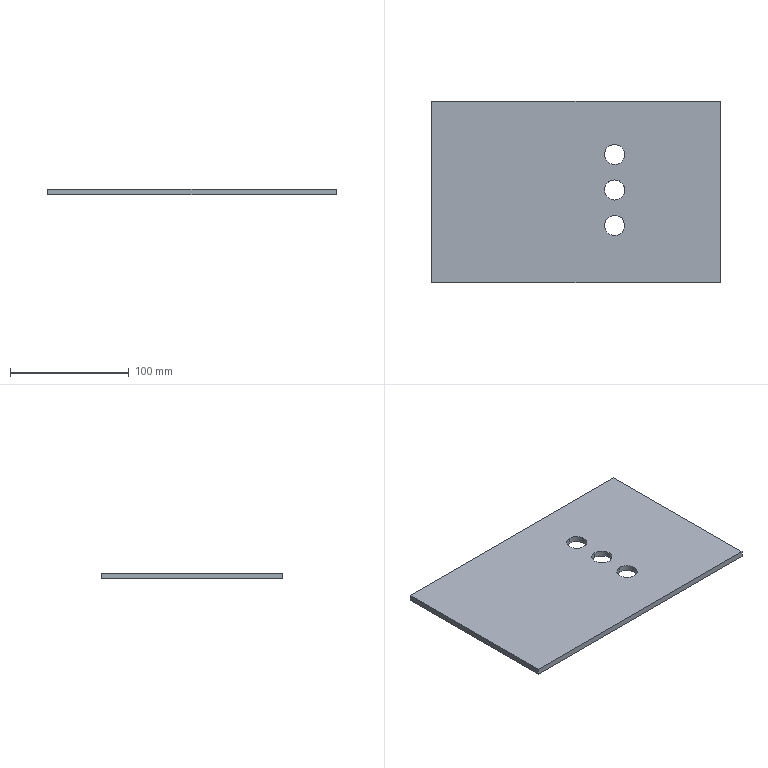Part | NX | features BREP 1 | 1 solid | 12 faces | box 243.374 x 152.848 x 5 mm | volume 182593 mm3 | cylinder 6 | plane 6 | commonest cylinder face diameters 17 x6
STEP:
#1=CARTESIAN_POINT('',(1894.999,-438.5,55.));
#2=VERTEX_POINT('',#1);
#3=CARTESIAN_POINT('',(1895.001,-421.5,55.));
#4=VERTEX_POINT('',#3);
#5=CARTESIAN_POINT('',(1895.,-438.5,55.));
#6=CARTESIAN_POINT('',(1895.974,-438.5,55.));
#7=CARTESIAN_POINT('',(1897.93,-438.172,55.));
#8=CARTESIAN_POINT('',(1901.646,-436.045,55.));
#9=CARTESIAN_POINT('',(1904.44,-430.737,55.));
#10=CARTESIAN_POINT('',(1902.023,-423.576,55.));
#11=CARTESIAN_POINT('',(1897.362,-421.5,55.));
#12=CARTESIAN_POINT('',(1895.001,-421.5,55.));
#13=B_SPLINE_CURVE_WITH_KNOTS('',3,(#5,#6,#7,#8,#9,#10,#11,#12),.UNSPECIFIED.,.F.,.F.,(4,1,1,1,1,4),(0.,0.125,0.25,0.5,0.75,1.),.UNSPECIFIED.);
#14=EDGE_CURVE('',#2,#4,#13,.T.);
#15=ORIENTED_EDGE('',*,*,#14,.F.);
#16=CARTESIAN_POINT('',(1895.001,-438.5,60.));
#17=VERTEX_POINT('',#16);
#18=CARTESIAN_POINT('',(1895.,-438.5,55.));
#19=CARTESIAN_POINT('',(1895.,-438.5,56.));
#20=CARTESIAN_POINT('',(1895.,-438.5,57.));
#21=CARTESIAN_POINT('',(1895.,-438.5,58.));
#22=CARTESIAN_POINT('',(1895.,-438.5,59.));
#23=CARTESIAN_POINT('',(1895.,-438.5,60.));
#24=(BOUNDED_CURVE()B_SPLINE_CURVE(5,(#18,#19,#20,#21,#22,#23),.UNSPECIFIED.,.F.,.F.)B_SPLINE_CURVE_WITH_KNOTS((6,6),(106.,111.),.UNSPECIFIED.)CURVE()GEOMETRIC_REPRESENTATION_ITEM()RATIONAL_B_SPLINE_CURVE((1.,1.,1.,1.,1.,1.))REPRESENTATION_ITEM(''));
#25=EDGE_CURVE('',#2,#17,#24,.T.);
#26=ORIENTED_EDGE('',*,*,#25,.T.);
#27=CARTESIAN_POINT('',(1894.999,-421.5,60.));
#28=VERTEX_POINT('',#27);
#29=CARTESIAN_POINT('',(1895.,-421.5,60.));
#30=CARTESIAN_POINT('',(1897.359,-421.5,60.));
#31=CARTESIAN_POINT('',(1902.023,-423.576,60.));
#32=CARTESIAN_POINT('',(1904.44,-430.736,60.));
#33=CARTESIAN_POINT('',(1901.647,-436.044,60.));
#34=CARTESIAN_POINT('',(1897.931,-438.171,60.));
#35=CARTESIAN_POINT('',(1895.976,-438.5,60.));
#36=CARTESIAN_POINT('',(1895.001,-438.5,60.));
#37=B_SPLINE_CURVE_WITH_KNOTS('',3,(#29,#30,#31,#32,#33,#34,#35,#36),.UNSPECIFIED.,.F.,.F.,(4,1,1,1,1,4),(0.,0.25,0.5,0.75,0.875,1.),.UNSPECIFIED.);
#38=EDGE_CURVE('',#17,#28,#37,.F.);
#39=ORIENTED_EDGE('',*,*,#38,.T.);
#40=CARTESIAN_POINT('',(1895.,-421.5,55.));
#41=CARTESIAN_POINT('',(1895.,-421.5,56.));
#42=CARTESIAN_POINT('',(1895.,-421.5,57.));
#43=CARTESIAN_POINT('',(1895.,-421.5,58.));
#44=CARTESIAN_POINT('',(1895.,-421.5,59.));
#45=CARTESIAN_POINT('',(1895.,-421.5,60.));
#46=(BOUNDED_CURVE()B_SPLINE_CURVE(5,(#40,#41,#42,#43,#44,#45),.UNSPECIFIED.,.F.,.F.)B_SPLINE_CURVE_WITH_KNOTS((6,6),(106.,111.),.UNSPECIFIED.)CURVE()GEOMETRIC_REPRESENTATION_ITEM()RATIONAL_B_SPLINE_CURVE((0.25,0.25,0.25,0.25,0.25,0.25))REPRESENTATION_ITEM(''));
#47=EDGE_CURVE('',#4,#28,#46,.T.);
#48=ORIENTED_EDGE('',*,*,#47,.F.);
#49=EDGE_LOOP('',(#15,#26,#39,#48));
#50=FACE_BOUND('',#49,.T.);
#51=CARTESIAN_POINT('',(1895.,-430.,49.));
#52=DIRECTION('',(0.,0.,1.));
#53=DIRECTION('',(1.,0.,0.));
#54=AXIS2_PLACEMENT_3D('',#51,#52,#53);
#55=CYLINDRICAL_SURFACE('',#54,8.5);
#56=ADVANCED_FACE('',(#50),#55,.F.);
#57=CARTESIAN_POINT('',(1895.,-421.5,55.));
#58=CARTESIAN_POINT('',(1892.641,-421.5,55.));
#59=CARTESIAN_POINT('',(1887.977,-423.575,55.));
#60=CARTESIAN_POINT('',(1885.56,-430.735,55.));
#61=CARTESIAN_POINT('',(1888.352,-436.043,55.));
#62=CARTESIAN_POINT('',(1892.069,-438.171,55.));
#63=CARTESIAN_POINT('',(1894.024,-438.5,55.));
#64=CARTESIAN_POINT('',(1894.999,-438.5,55.));
#65=B_SPLINE_CURVE_WITH_KNOTS('',3,(#57,#58,#59,#60,#61,#62,#63,#64),.UNSPECIFIED.,.F.,.F.,(4,1,1,1,1,4),(0.,0.25,0.5,0.75,0.875,1.),.UNSPECIFIED.);
#66=EDGE_CURVE('',#4,#2,#65,.T.);
#67=ORIENTED_EDGE('',*,*,#66,.F.);
#68=ORIENTED_EDGE('',*,*,#47,.T.);
#69=CARTESIAN_POINT('',(1895.,-438.5,60.));
#70=CARTESIAN_POINT('',(1894.026,-438.5,60.));
#71=CARTESIAN_POINT('',(1892.069,-438.172,60.));
#72=CARTESIAN_POINT('',(1888.353,-436.044,60.));
#73=CARTESIAN_POINT('',(1885.56,-430.737,60.));
#74=CARTESIAN_POINT('',(1887.977,-423.576,60.));
#75=CARTESIAN_POINT('',(1892.639,-421.5,60.));
#76=CARTESIAN_POINT('',(1894.999,-421.5,60.));
#77=B_SPLINE_CURVE_WITH_KNOTS('',3,(#69,#70,#71,#72,#73,#74,#75,#76),.UNSPECIFIED.,.F.,.F.,(4,1,1,1,1,4),(0.,0.125,0.25,0.5,0.75,1.),.UNSPECIFIED.);
#78=EDGE_CURVE('',#28,#17,#77,.F.);
#79=ORIENTED_EDGE('',*,*,#78,.T.);
#80=ORIENTED_EDGE('',*,*,#25,.F.);
#81=EDGE_LOOP('',(#67,#68,#79,#80));
#82=FACE_BOUND('',#81,.T.);
#83=CARTESIAN_POINT('',(1895.,-430.,49.));
#84=DIRECTION('',(0.,0.,1.));
#85=DIRECTION('',(0.,-1.,0.));
#86=AXIS2_PLACEMENT_3D('',#83,#84,#85);
#87=CYLINDRICAL_SURFACE('',#86,8.5);
#88=ADVANCED_FACE('',(#82),#87,.F.);
#89=CARTESIAN_POINT('',(1894.999,-468.5,55.));
#90=VERTEX_POINT('',#89);
#91=CARTESIAN_POINT('',(1895.001,-451.5,55.));
#92=VERTEX_POINT('',#91);
#93=CARTESIAN_POINT('',(1895.,-468.5,55.));
#94=CARTESIAN_POINT('',(1895.974,-468.5,55.));
#95=CARTESIAN_POINT('',(1897.93,-468.172,55.));
#96=CARTESIAN_POINT('',(1901.646,-466.045,55.));
#97=CARTESIAN_POINT('',(1904.44,-460.737,55.));
#98=CARTESIAN_POINT('',(1902.023,-453.576,55.));
#99=CARTESIAN_POINT('',(1897.362,-451.5,55.));
#100=CARTESIAN_POINT('',(1895.001,-451.5,55.));
#101=B_SPLINE_CURVE_WITH_KNOTS('',3,(#93,#94,#95,#96,#97,#98,#99,#100),.UNSPECIFIED.,.F.,.F.,(4,1,1,1,1,4),(0.,0.125,0.25,0.5,0.75,1.),.UNSPECIFIED.);
#102=EDGE_CURVE('',#90,#92,#101,.T.);
#103=ORIENTED_EDGE('',*,*,#102,.F.);
#104=CARTESIAN_POINT('',(1895.001,-468.5,60.));
#105=VERTEX_POINT('',#104);
#106=CARTESIAN_POINT('',(1895.,-468.5,55.));
#107=CARTESIAN_POINT('',(1895.,-468.5,56.));
#108=CARTESIAN_POINT('',(1895.,-468.5,57.));
#109=CARTESIAN_POINT('',(1895.,-468.5,58.));
#110=CARTESIAN_POINT('',(1895.,-468.5,59.));
#111=CARTESIAN_POINT('',(1895.,-468.5,60.));
#112=(BOUNDED_CURVE()B_SPLINE_CURVE(5,(#106,#107,#108,#109,#110,#111),.UNSPECIFIED.,.F.,.F.)B_SPLINE_CURVE_WITH_KNOTS((6,6),(106.,111.),.UNSPECIFIED.)CURVE()GEOMETRIC_REPRESENTATION_ITEM()RATIONAL_B_SPLINE_CURVE((1.,1.,1.,1.,1.,1.))REPRESENTATION_ITEM(''));
#113=EDGE_CURVE('',#90,#105,#112,.T.);
#114=ORIENTED_EDGE('',*,*,#113,.T.);
#115=CARTESIAN_POINT('',(1894.999,-451.5,60.));
#116=VERTEX_POINT('',#115);
#117=CARTESIAN_POINT('',(1895.,-451.5,60.));
#118=CARTESIAN_POINT('',(1897.359,-451.5,60.));
#119=CARTESIAN_POINT('',(1902.023,-453.576,60.));
#120=CARTESIAN_POINT('',(1904.44,-460.736,60.));
#121=CARTESIAN_POINT('',(1901.647,-466.044,60.));
#122=CARTESIAN_POINT('',(1897.931,-468.171,60.));
#123=CARTESIAN_POINT('',(1895.976,-468.5,60.));
#124=CARTESIAN_POINT('',(1895.001,-468.5,60.));
#125=B_SPLINE_CURVE_WITH_KNOTS('',3,(#117,#118,#119,#120,#121,#122,#123,#124),.UNSPECIFIED.,.F.,.F.,(4,1,1,1,1,4),(0.,0.25,0.5,0.75,0.875,1.),.UNSPECIFIED.);
#126=EDGE_CURVE('',#105,#116,#125,.F.);
#127=ORIENTED_EDGE('',*,*,#126,.T.);
#128=CARTESIAN_POINT('',(1895.,-451.5,55.));
#129=CARTESIAN_POINT('',(1895.,-451.5,56.));
#130=CARTESIAN_POINT('',(1895.,-451.5,57.));
#131=CARTESIAN_POINT('',(1895.,-451.5,58.));
#132=CARTESIAN_POINT('',(1895.,-451.5,59.));
#133=CARTESIAN_POINT('',(1895.,-451.5,60.));
#134=(BOUNDED_CURVE()B_SPLINE_CURVE(5,(#128,#129,#130,#131,#132,#133),.UNSPECIFIED.,.F.,.F.)B_SPLINE_CURVE_WITH_KNOTS((6,6),(106.,111.),.UNSPECIFIED.)CURVE()GEOMETRIC_REPRESENTATION_ITEM()RATIONAL_B_SPLINE_CURVE((0.25,0.25,0.25,0.25,0.25,0.25))REPRESENTATION_ITEM(''));
#135=EDGE_CURVE('',#92,#116,#134,.T.);
#136=ORIENTED_EDGE('',*,*,#135,.F.);
#137=EDGE_LOOP('',(#103,#114,#127,#136));
#138=FACE_BOUND('',#137,.T.);
#139=CARTESIAN_POINT('',(1895.,-460.,49.));
#140=DIRECTION('',(0.,0.,1.));
#141=DIRECTION('',(1.,0.,0.));
#142=AXIS2_PLACEMENT_3D('',#139,#140,#141);
#143=CYLINDRICAL_SURFACE('',#142,8.5);
#144=ADVANCED_FACE('',(#138),#143,.F.);
#145=CARTESIAN_POINT('',(1895.,-451.5,55.));
#146=CARTESIAN_POINT('',(1892.641,-451.5,55.));
#147=CARTESIAN_POINT('',(1887.977,-453.575,55.));
#148=CARTESIAN_POINT('',(1885.56,-460.735,55.));
#149=CARTESIAN_POINT('',(1888.352,-466.043,55.));
#150=CARTESIAN_POINT('',(1892.069,-468.171,55.));
#151=CARTESIAN_POINT('',(1894.024,-468.5,55.));
#152=CARTESIAN_POINT('',(1894.999,-468.5,55.));
#153=B_SPLINE_CURVE_WITH_KNOTS('',3,(#145,#146,#147,#148,#149,#150,#151,#152),.UNSPECIFIED.,.F.,.F.,(4,1,1,1,1,4),(0.,0.25,0.5,0.75,0.875,1.),.UNSPECIFIED.);
#154=EDGE_CURVE('',#92,#90,#153,.T.);
#155=ORIENTED_EDGE('',*,*,#154,.F.);
#156=ORIENTED_EDGE('',*,*,#135,.T.);
#157=CARTESIAN_POINT('',(1895.,-468.5,60.));
#158=CARTESIAN_POINT('',(1894.026,-468.5,60.));
#159=CARTESIAN_POINT('',(1892.069,-468.172,60.));
#160=CARTESIAN_POINT('',(1888.353,-466.044,60.));
#161=CARTESIAN_POINT('',(1885.56,-460.737,60.));
#162=CARTESIAN_POINT('',(1887.977,-453.576,60.));
#163=CARTESIAN_POINT('',(1892.639,-451.5,60.));
#164=CARTESIAN_POINT('',(1894.999,-451.5,60.));
#165=B_SPLINE_CURVE_WITH_KNOTS('',3,(#157,#158,#159,#160,#161,#162,#163,#164),.UNSPECIFIED.,.F.,.F.,(4,1,1,1,1,4),(0.,0.125,0.25,0.5,0.75,1.),.UNSPECIFIED.);
#166=EDGE_CURVE('',#116,#105,#165,.F.);
#167=ORIENTED_EDGE('',*,*,#166,.T.);
#168=ORIENTED_EDGE('',*,*,#113,.F.);
#169=EDGE_LOOP('',(#155,#156,#167,#168));
#170=FACE_BOUND('',#169,.T.);
#171=CARTESIAN_POINT('',(1895.,-460.,49.));
#172=DIRECTION('',(0.,0.,1.));
#173=DIRECTION('',(0.,-1.,0.));
#174=AXIS2_PLACEMENT_3D('',#171,#172,#173);
#175=CYLINDRICAL_SURFACE('',#174,8.5);
#176=ADVANCED_FACE('',(#170),#175,.F.);
#177=CARTESIAN_POINT('',(1894.999,-498.5,55.));
#178=VERTEX_POINT('',#177);
#179=CARTESIAN_POINT('',(1895.001,-481.5,55.));
#180=VERTEX_POINT('',#179);
#181=CARTESIAN_POINT('',(1895.,-498.5,55.));
#182=CARTESIAN_POINT('',(1895.974,-498.5,55.));
#183=CARTESIAN_POINT('',(1897.93,-498.172,55.));
#184=CARTESIAN_POINT('',(1901.646,-496.045,55.));
#185=CARTESIAN_POINT('',(1904.44,-490.737,55.));
#186=CARTESIAN_POINT('',(1902.023,-483.576,55.));
#187=CARTESIAN_POINT('',(1897.362,-481.5,55.));
#188=CARTESIAN_POINT('',(1895.001,-481.5,55.));
#189=B_SPLINE_CURVE_WITH_KNOTS('',3,(#181,#182,#183,#184,#185,#186,#187,#188),.UNSPECIFIED.,.F.,.F.,(4,1,1,1,1,4),(0.,0.125,0.25,0.5,0.75,1.),.UNSPECIFIED.);
#190=EDGE_CURVE('',#178,#180,#189,.T.);
#191=ORIENTED_EDGE('',*,*,#190,.F.);
#192=CARTESIAN_POINT('',(1895.,-498.5,60.));
#193=VERTEX_POINT('',#192);
#194=CARTESIAN_POINT('',(1895.,-498.5,55.));
#195=CARTESIAN_POINT('',(1895.,-498.5,56.));
#196=CARTESIAN_POINT('',(1895.,-498.5,57.));
#197=CARTESIAN_POINT('',(1895.,-498.5,58.));
#198=CARTESIAN_POINT('',(1895.,-498.5,59.));
#199=CARTESIAN_POINT('',(1895.,-498.5,60.));
#200=(BOUNDED_CURVE()B_SPLINE_CURVE(5,(#194,#195,#196,#197,#198,#199),.UNSPECIFIED.,.F.,.F.)B_SPLINE_CURVE_WITH_KNOTS((6,6),(106.,111.),.UNSPECIFIED.)CURVE()GEOMETRIC_REPRESENTATION_ITEM()RATIONAL_B_SPLINE_CURVE((1.,1.,1.,1.,1.,1.))REPRESENTATION_ITEM(''));
#201=EDGE_CURVE('',#178,#193,#200,.T.);
#202=ORIENTED_EDGE('',*,*,#201,.T.);
#203=CARTESIAN_POINT('',(1895.,-481.5,60.));
#204=VERTEX_POINT('',#203);
#205=CARTESIAN_POINT('',(1895.,-498.5,60.));
#206=CARTESIAN_POINT('',(1895.807,-498.5,60.));
#207=CARTESIAN_POINT('',(1896.636,-498.404,60.));
#208=CARTESIAN_POINT('',(1897.469,-498.202,60.));
#209=CARTESIAN_POINT('',(1899.048,-497.596,60.));
#210=CARTESIAN_POINT('',(1900.474,-496.585,60.));
#211=CARTESIAN_POINT('',(1901.109,-496.004,60.));
#212=CARTESIAN_POINT('',(1902.209,-494.702,60.));
#213=CARTESIAN_POINT('',(1902.968,-493.138,60.));
#214=CARTESIAN_POINT('',(1903.245,-492.321,60.));
#215=CARTESIAN_POINT('',(1903.584,-490.642,60.));
#216=CARTESIAN_POINT('',(1903.495,-488.91,60.));
#217=CARTESIAN_POINT('',(1903.343,-488.06,60.));
#218=CARTESIAN_POINT('',(1902.828,-486.42,60.));
#219=CARTESIAN_POINT('',(1901.916,-484.948,60.));
#220=CARTESIAN_POINT('',(1901.371,-484.276,60.));
#221=CARTESIAN_POINT('',(1900.125,-483.084,60.));
#222=CARTESIAN_POINT('',(1898.617,-482.236,60.));
#223=CARTESIAN_POINT('',(1897.815,-481.911,60.));
#224=CARTESIAN_POINT('',(1896.759,-481.631,60.));
#225=CARTESIAN_POINT('',(1895.679,-481.523,60.));
#226=CARTESIAN_POINT('',(1895.453,-481.508,60.));
#227=CARTESIAN_POINT('',(1895.227,-481.5,60.));
#228=CARTESIAN_POINT('',(1895.,-481.5,60.));
#229=B_SPLINE_CURVE_WITH_KNOTS('',5,(#205,#206,#207,#208,#209,#210,#211,#212,#213,#214,#215,#216,#217,#218,#219,#220,#221,#222,#223,#224,#225,#226,#227,#228),.UNSPECIFIED.,.F.,.F.,(6,3,3,3,3,3,3,6),(0.,6.667,12.918,18.932,24.809,30.609,36.373,37.896),.UNSPECIFIED.);
#230=EDGE_CURVE('',#193,#204,#229,.T.);
#231=ORIENTED_EDGE('',*,*,#230,.T.);
#232=CARTESIAN_POINT('',(1895.,-481.5,55.));
#233=CARTESIAN_POINT('',(1895.,-481.5,56.));
#234=CARTESIAN_POINT('',(1895.,-481.5,57.));
#235=CARTESIAN_POINT('',(1895.,-481.5,58.));
#236=CARTESIAN_POINT('',(1895.,-481.5,59.));
#237=CARTESIAN_POINT('',(1895.,-481.5,60.));
#238=(BOUNDED_CURVE()B_SPLINE_CURVE(5,(#232,#233,#234,#235,#236,#237),.UNSPECIFIED.,.F.,.F.)B_SPLINE_CURVE_WITH_KNOTS((6,6),(106.,111.),.UNSPECIFIED.)CURVE()GEOMETRIC_REPRESENTATION_ITEM()RATIONAL_B_SPLINE_CURVE((0.25,0.25,0.25,0.25,0.25,0.25))REPRESENTATION_ITEM(''));
#239=EDGE_CURVE('',#180,#204,#238,.T.);
#240=ORIENTED_EDGE('',*,*,#239,.F.);
#241=EDGE_LOOP('',(#191,#202,#231,#240));
#242=FACE_BOUND('',#241,.T.);
#243=CARTESIAN_POINT('',(1895.,-490.,49.));
#244=DIRECTION('',(0.,0.,1.));
#245=DIRECTION('',(0.,-1.,0.));
#246=AXIS2_PLACEMENT_3D('',#243,#244,#245);
#247=CYLINDRICAL_SURFACE('',#246,8.5);
#248=ADVANCED_FACE('',(#242),#247,.F.);
#249=CARTESIAN_POINT('',(1895.,-481.5,55.));
#250=CARTESIAN_POINT('',(1892.641,-481.5,55.));
#251=CARTESIAN_POINT('',(1887.977,-483.575,55.));
#252=CARTESIAN_POINT('',(1885.56,-490.735,55.));
#253=CARTESIAN_POINT('',(1888.352,-496.043,55.));
#254=CARTESIAN_POINT('',(1892.069,-498.171,55.));
#255=CARTESIAN_POINT('',(1894.024,-498.5,55.));
#256=CARTESIAN_POINT('',(1894.999,-498.5,55.));
#257=B_SPLINE_CURVE_WITH_KNOTS('',3,(#249,#250,#251,#252,#253,#254,#255,#256),.UNSPECIFIED.,.F.,.F.,(4,1,1,1,1,4),(0.,0.25,0.5,0.75,0.875,1.),.UNSPECIFIED.);
#258=EDGE_CURVE('',#180,#178,#257,.T.);
#259=ORIENTED_EDGE('',*,*,#258,.F.);
#260=ORIENTED_EDGE('',*,*,#239,.T.);
#261=CARTESIAN_POINT('',(1895.,-498.5,60.));
#262=CARTESIAN_POINT('',(1894.024,-498.5,60.));
#263=CARTESIAN_POINT('',(1892.066,-498.171,60.));
#264=CARTESIAN_POINT('',(1888.348,-496.04,60.));
#265=CARTESIAN_POINT('',(1885.56,-490.728,60.));
#266=CARTESIAN_POINT('',(1887.982,-483.572,60.));
#267=CARTESIAN_POINT('',(1892.641,-481.5,60.));
#268=CARTESIAN_POINT('',(1895.,-481.5,60.));
#269=B_SPLINE_CURVE_WITH_KNOTS('',3,(#261,#262,#263,#264,#265,#266,#267,#268),.UNSPECIFIED.,.F.,.F.,(4,1,1,1,1,4),(0.,0.125,0.25,0.5,0.75,1.),.UNSPECIFIED.);
#270=EDGE_CURVE('',#204,#193,#269,.F.);
#271=ORIENTED_EDGE('',*,*,#270,.T.);
#272=ORIENTED_EDGE('',*,*,#201,.F.);
#273=EDGE_LOOP('',(#259,#260,#271,#272));
#274=FACE_BOUND('',#273,.T.);
#275=CARTESIAN_POINT('',(1895.,-490.,49.));
#276=DIRECTION('',(0.,0.,1.));
#277=DIRECTION('',(1.,0.,0.));
#278=AXIS2_PLACEMENT_3D('',#275,#276,#277);
#279=CYLINDRICAL_SURFACE('',#278,8.5);
#280=ADVANCED_FACE('',(#274),#279,.F.);
#281=CARTESIAN_POINT('',(1740.711,-385.283,55.));
#282=VERTEX_POINT('',#281);
#283=CARTESIAN_POINT('',(1740.711,-385.283,60.));
#284=VERTEX_POINT('',#283);
#285=CARTESIAN_POINT('',(1740.711,-385.283,57.5));
#286=DIRECTION('',(0.,0.,1.));
#287=VECTOR('',#286,1000.);
#288=LINE('',#285,#287);
#289=EDGE_CURVE('',#282,#284,#288,.T.);
#290=ORIENTED_EDGE('',*,*,#289,.F.);
#291=CARTESIAN_POINT('',(1740.711,-538.131,55.));
#292=VERTEX_POINT('',#291);
#293=CARTESIAN_POINT('',(1740.711,-461.707,55.));
#294=DIRECTION('',(0.,1.,0.));
#295=VECTOR('',#294,1000.);
#296=LINE('',#293,#295);
#297=EDGE_CURVE('',#292,#282,#296,.T.);
#298=ORIENTED_EDGE('',*,*,#297,.F.);
#299=CARTESIAN_POINT('',(1740.711,-538.131,60.));
#300=VERTEX_POINT('',#299);
#301=CARTESIAN_POINT('',(1740.711,-538.131,57.5));
#302=DIRECTION('',(0.,0.,1.));
#303=VECTOR('',#302,1000.);
#304=LINE('',#301,#303);
#305=EDGE_CURVE('',#292,#300,#304,.T.);
#306=ORIENTED_EDGE('',*,*,#305,.T.);
#307=CARTESIAN_POINT('',(1740.711,-461.707,60.));
#308=DIRECTION('',(0.,1.,0.));
#309=VECTOR('',#308,1000.);
#310=LINE('',#307,#309);
#311=EDGE_CURVE('',#300,#284,#310,.T.);
#312=ORIENTED_EDGE('',*,*,#311,.T.);
#313=EDGE_LOOP('',(#290,#298,#306,#312));
#314=FACE_BOUND('',#313,.T.);
#315=CARTESIAN_POINT('',(1740.711,-461.707,60.));
#316=DIRECTION('',(1.,0.,0.));
#317=DIRECTION('',(0.,1.,0.));
#318=AXIS2_PLACEMENT_3D('',#315,#316,#317);
#319=PLANE('',#318);
#320=ADVANCED_FACE('',(#314),#319,.F.);
#321=ORIENTED_EDGE('',*,*,#305,.F.);
#322=CARTESIAN_POINT('',(1984.086,-538.131,55.));
#323=VERTEX_POINT('',#322);
#324=CARTESIAN_POINT('',(1862.398,-538.131,55.));
#325=DIRECTION('',(1.,0.,0.));
#326=VECTOR('',#325,1000.);
#327=LINE('',#324,#326);
#328=EDGE_CURVE('',#292,#323,#327,.T.);
#329=ORIENTED_EDGE('',*,*,#328,.T.);
#330=CARTESIAN_POINT('',(1984.086,-538.131,60.));
#331=VERTEX_POINT('',#330);
#332=CARTESIAN_POINT('',(1984.086,-538.131,57.5));
#333=DIRECTION('',(0.,0.,-1.));
#334=VECTOR('',#333,1000.);
#335=LINE('',#332,#334);
#336=EDGE_CURVE('',#331,#323,#335,.T.);
#337=ORIENTED_EDGE('',*,*,#336,.F.);
#338=CARTESIAN_POINT('',(1862.398,-538.131,60.));
#339=DIRECTION('',(1.,0.,0.));
#340=VECTOR('',#339,1000.);
#341=LINE('',#338,#340);
#342=EDGE_CURVE('',#300,#331,#341,.T.);
#343=ORIENTED_EDGE('',*,*,#342,.F.);
#344=EDGE_LOOP('',(#321,#329,#337,#343));
#345=FACE_BOUND('',#344,.T.);
#346=CARTESIAN_POINT('',(1867.043,-538.131,60.));
#347=DIRECTION('',(0.,-1.,0.));
#348=DIRECTION('',(1.,0.,0.));
#349=AXIS2_PLACEMENT_3D('',#346,#347,#348);
#350=PLANE('',#349);
#351=ADVANCED_FACE('',(#345),#350,.T.);
#352=ORIENTED_EDGE('',*,*,#38,.F.);
#353=ORIENTED_EDGE('',*,*,#78,.F.);
#354=EDGE_LOOP('',(#352,#353));
#355=FACE_BOUND('',#354,.T.);
#356=ORIENTED_EDGE('',*,*,#126,.F.);
#357=ORIENTED_EDGE('',*,*,#166,.F.);
#358=EDGE_LOOP('',(#356,#357));
#359=FACE_BOUND('',#358,.T.);
#360=ORIENTED_EDGE('',*,*,#230,.F.);
#361=ORIENTED_EDGE('',*,*,#270,.F.);
#362=EDGE_LOOP('',(#360,#361));
#363=FACE_BOUND('',#362,.T.);
#364=ORIENTED_EDGE('',*,*,#342,.T.);
#365=CARTESIAN_POINT('',(1984.086,-385.283,60.));
#366=VERTEX_POINT('',#365);
#367=CARTESIAN_POINT('',(1984.086,-461.707,60.));
#368=DIRECTION('',(0.,1.,0.));
#369=VECTOR('',#368,1000.);
#370=LINE('',#367,#369);
#371=EDGE_CURVE('',#331,#366,#370,.T.);
#372=ORIENTED_EDGE('',*,*,#371,.T.);
#373=CARTESIAN_POINT('',(1862.398,-385.283,60.));
#374=DIRECTION('',(1.,0.,0.));
#375=VECTOR('',#374,1000.);
#376=LINE('',#373,#375);
#377=EDGE_CURVE('',#284,#366,#376,.T.);
#378=ORIENTED_EDGE('',*,*,#377,.F.);
#379=ORIENTED_EDGE('',*,*,#311,.F.);
#380=EDGE_LOOP('',(#364,#372,#378,#379));
#381=FACE_BOUND('',#380,.T.);
#382=CARTESIAN_POINT('',(0.,0.,60.));
#383=DIRECTION('',(0.,0.,-1.));
#384=DIRECTION('',(1.,0.,0.));
#385=AXIS2_PLACEMENT_3D('',#382,#383,#384);
#386=PLANE('',#385);
#387=ADVANCED_FACE('',(#355,#359,#363,#381),#386,.F.);
#388=ORIENTED_EDGE('',*,*,#377,.T.);
#389=CARTESIAN_POINT('',(1984.086,-385.283,55.));
#390=VERTEX_POINT('',#389);
#391=CARTESIAN_POINT('',(1984.086,-385.283,57.5));
#392=DIRECTION('',(0.,0.,-1.));
#393=VECTOR('',#392,1000.);
#394=LINE('',#391,#393);
#395=EDGE_CURVE('',#366,#390,#394,.T.);
#396=ORIENTED_EDGE('',*,*,#395,.T.);
#397=CARTESIAN_POINT('',(1862.398,-385.283,55.));
#398=DIRECTION('',(1.,0.,0.));
#399=VECTOR('',#398,1000.);
#400=LINE('',#397,#399);
#401=EDGE_CURVE('',#282,#390,#400,.T.);
#402=ORIENTED_EDGE('',*,*,#401,.F.);
#403=ORIENTED_EDGE('',*,*,#289,.T.);
#404=EDGE_LOOP('',(#388,#396,#402,#403));
#405=FACE_BOUND('',#404,.T.);
#406=CARTESIAN_POINT('',(1867.043,-385.283,60.));
#407=DIRECTION('',(0.,1.,0.));
#408=DIRECTION('',(1.,0.,0.));
#409=AXIS2_PLACEMENT_3D('',#406,#407,#408);
#410=PLANE('',#409);
#411=ADVANCED_FACE('',(#405),#410,.T.);
#412=ORIENTED_EDGE('',*,*,#66,.T.);
#413=ORIENTED_EDGE('',*,*,#14,.T.);
#414=EDGE_LOOP('',(#412,#413));
#415=FACE_BOUND('',#414,.T.);
#416=ORIENTED_EDGE('',*,*,#154,.T.);
#417=ORIENTED_EDGE('',*,*,#102,.T.);
#418=EDGE_LOOP('',(#416,#417));
#419=FACE_BOUND('',#418,.T.);
#420=ORIENTED_EDGE('',*,*,#258,.T.);
#421=ORIENTED_EDGE('',*,*,#190,.T.);
#422=EDGE_LOOP('',(#420,#421));
#423=FACE_BOUND('',#422,.T.);
#424=ORIENTED_EDGE('',*,*,#297,.T.);
#425=ORIENTED_EDGE('',*,*,#401,.T.);
#426=CARTESIAN_POINT('',(1984.086,-461.707,55.));
#427=DIRECTION('',(0.,1.,0.));
#428=VECTOR('',#427,1000.);
#429=LINE('',#426,#428);
#430=EDGE_CURVE('',#323,#390,#429,.T.);
#431=ORIENTED_EDGE('',*,*,#430,.F.);
#432=ORIENTED_EDGE('',*,*,#328,.F.);
#433=EDGE_LOOP('',(#424,#425,#431,#432));
#434=FACE_BOUND('',#433,.T.);
#435=CARTESIAN_POINT('',(0.,0.,55.));
#436=DIRECTION('',(0.,0.,-1.));
#437=DIRECTION('',(1.,0.,0.));
#438=AXIS2_PLACEMENT_3D('',#435,#436,#437);
#439=PLANE('',#438);
#440=ADVANCED_FACE('',(#415,#419,#423,#434),#439,.T.);
#441=ORIENTED_EDGE('',*,*,#430,.T.);
#442=ORIENTED_EDGE('',*,*,#395,.F.);
#443=ORIENTED_EDGE('',*,*,#371,.F.);
#444=ORIENTED_EDGE('',*,*,#336,.T.);
#445=EDGE_LOOP('',(#441,#442,#443,#444));
#446=FACE_BOUND('',#445,.T.);
#447=CARTESIAN_POINT('',(1984.086,-461.707,60.));
#448=DIRECTION('',(-1.,0.,0.));
#449=DIRECTION('',(0.,1.,0.));
#450=AXIS2_PLACEMENT_3D('',#447,#448,#449);
#451=PLANE('',#450);
#452=ADVANCED_FACE('',(#446),#451,.F.);
#453=CLOSED_SHELL('',(#56,#88,#144,#176,#248,#280,#320,#351,#387,#411,#440,#452));
#454=MANIFOLD_SOLID_BREP('',#453);
#455=(LENGTH_UNIT()NAMED_UNIT(*)SI_UNIT(.MILLI.,.METRE.));
#456=UNCERTAINTY_MEASURE_WITH_UNIT(LENGTH_MEASURE(0.0508),#455,'','');
#457=(NAMED_UNIT(*)PLANE_ANGLE_UNIT()SI_UNIT($,.RADIAN.));
#458=(NAMED_UNIT(*)SI_UNIT($,.STERADIAN.)SOLID_ANGLE_UNIT());
#459=(GEOMETRIC_REPRESENTATION_CONTEXT(3)GLOBAL_UNCERTAINTY_ASSIGNED_CONTEXT((#456))GLOBAL_UNIT_ASSIGNED_CONTEXT((#455,#457,#458))REPRESENTATION_CONTEXT('',''));
#460=ADVANCED_BREP_SHAPE_REPRESENTATION('',(#454),#459);